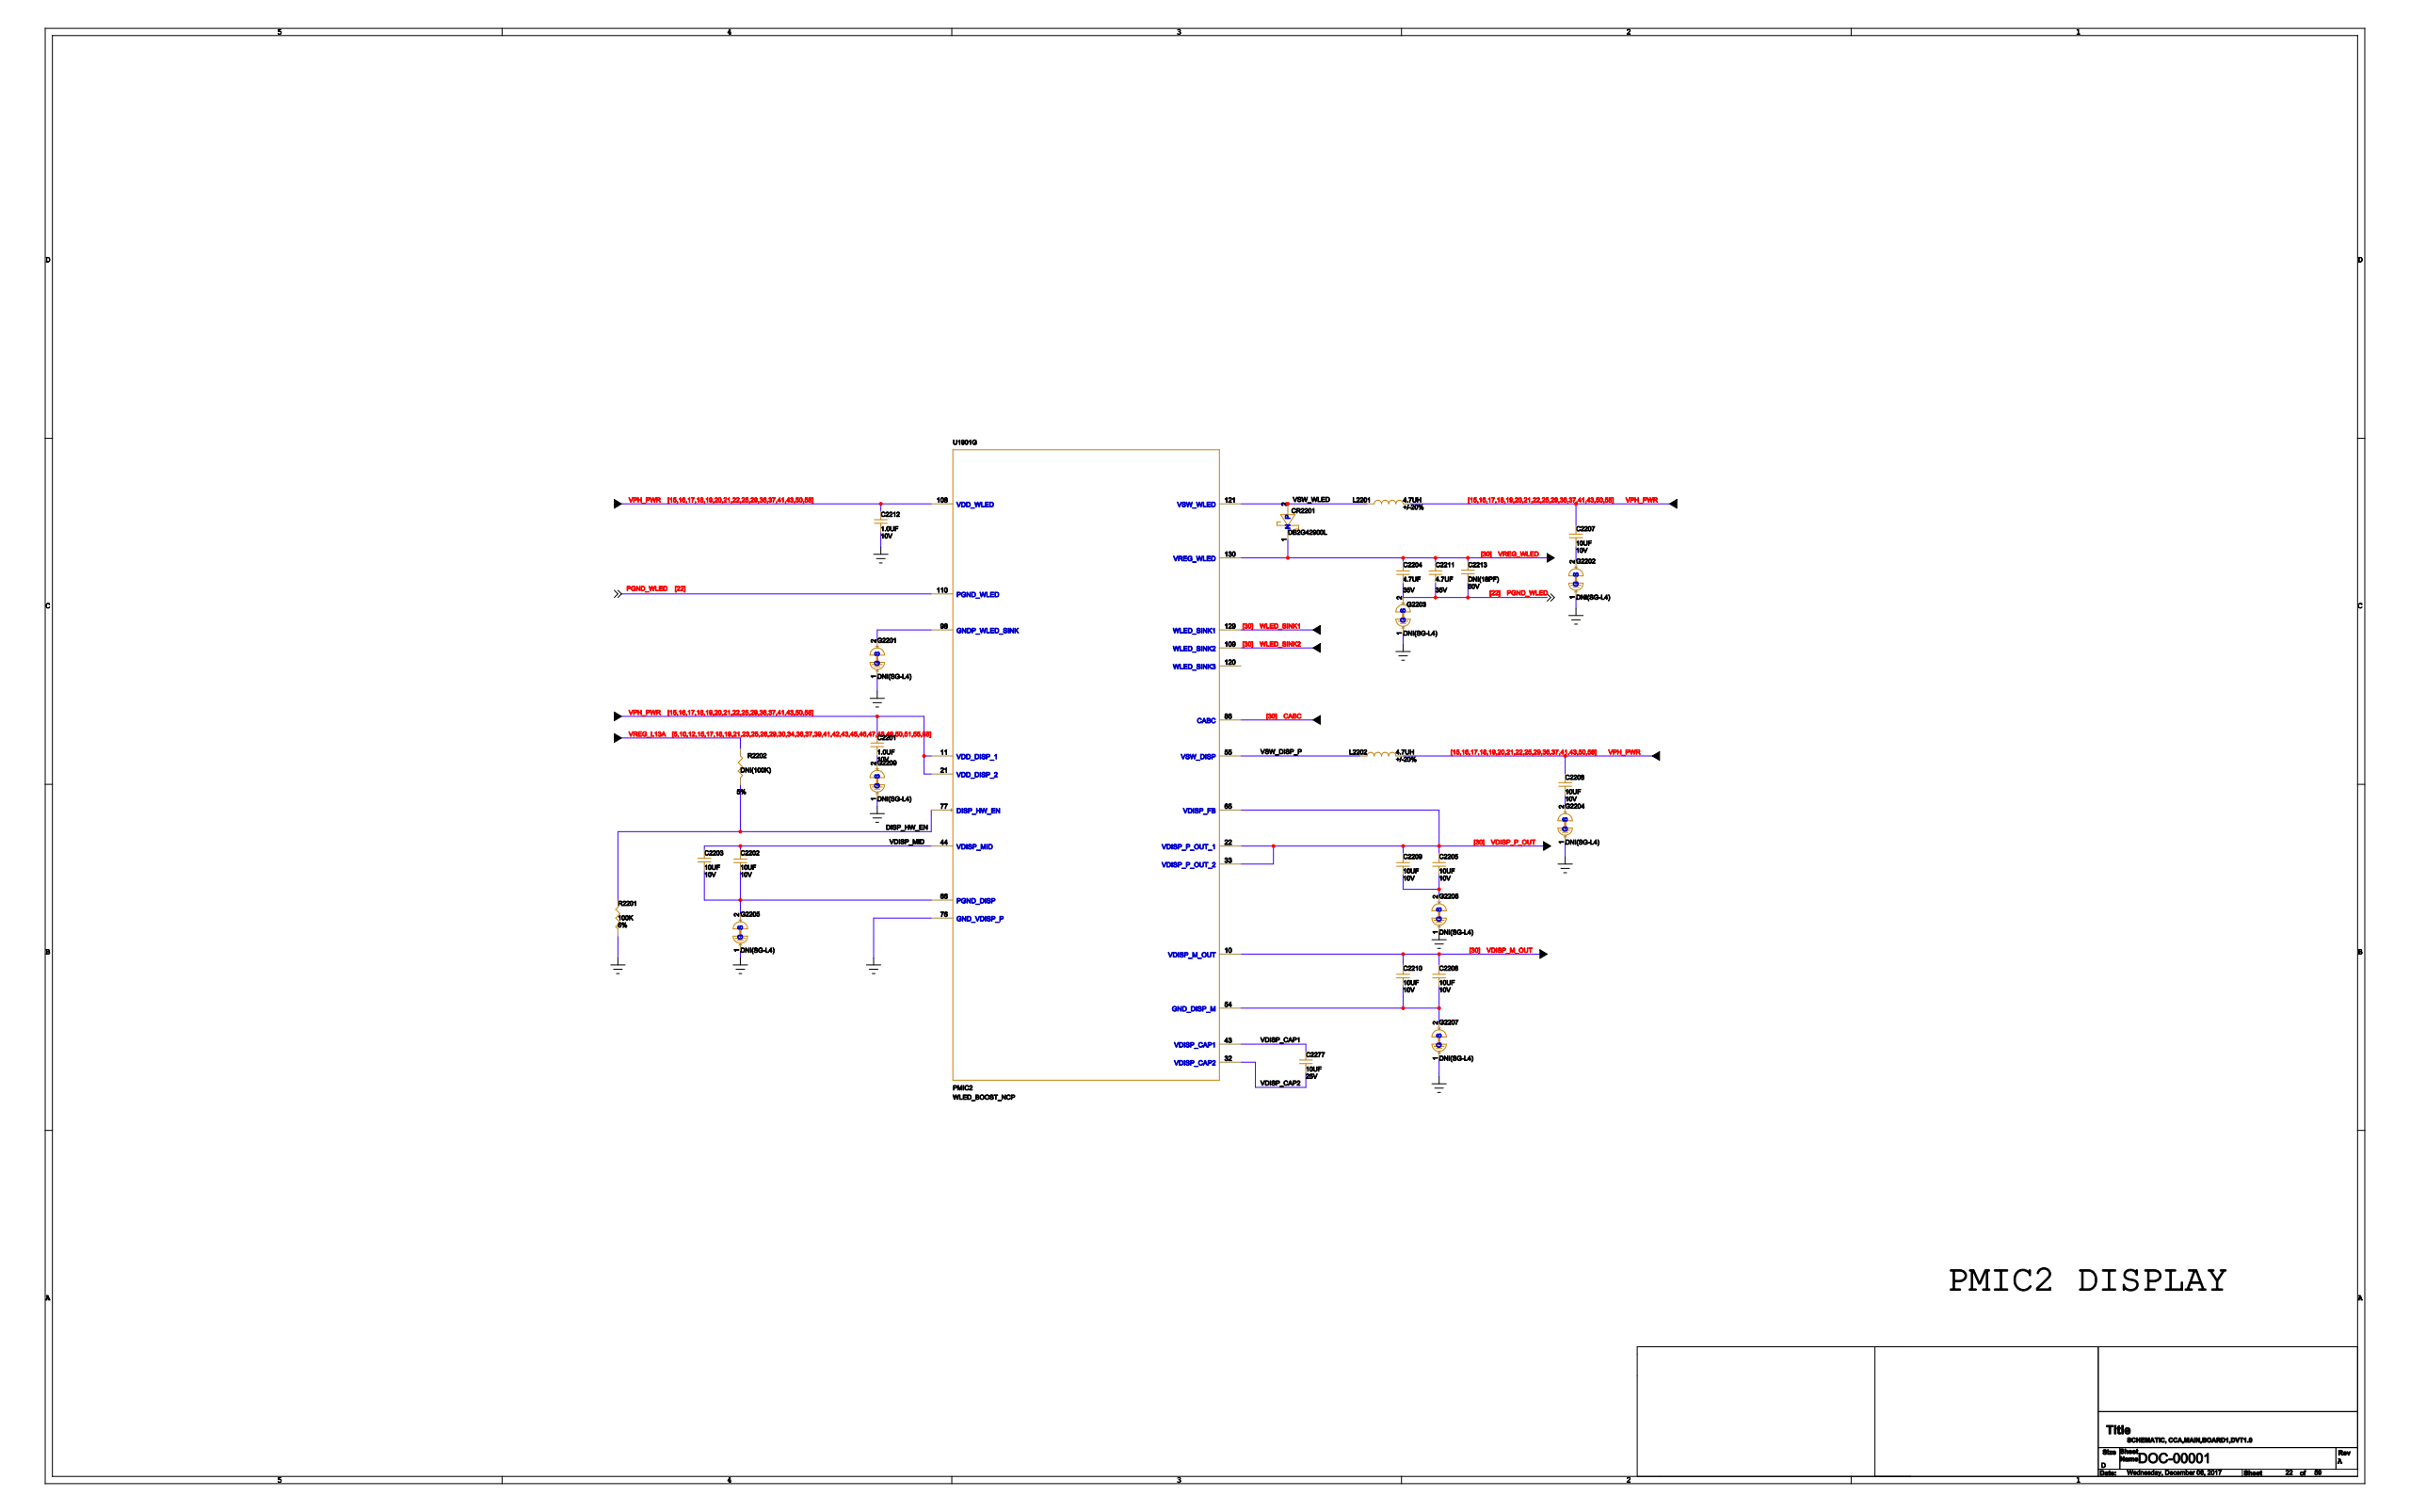Circuit board | KiCad | 1657 parts | 1365 nets | one sheet of the schematic
Parts on this sheet (reference | value | footprint):
C2201
C2202
C2203
C2204
C2205
C2206
C2207
C2208
C2209
C2210
C2211
C2212
C2213
C2277
CR2201
G2201
G2202
G2203
G2204
G2205
G2207
G2208
G2209
L2201
L2202
R2201
R2202
U1901
Nets of these parts (net: part-pin ...):
GND: C2212-2 G2201-1 G2202-1 G2203-1 G2204-1 G2205-1 G2207-1 G2208-1 G2209-1 R2201-2 U1901-76
VREG_L13A: R2202-2
VPH_PWR: C2201-1 C2207-1 C2208-1 C2212-1 L2201-2 L2202-2 U1901-2 U1901-11 U1901-17 U1901-21 U1901-39 U1901-108
N42480060: C2208-2 G2204-2
N42479215: G2201-2 U1901-98
CABC: U1901-86
N48943271: C2201-2 G2209-2
N48942883: C2205-1 C2209-1 G2208-2
PGND_WLED: C2204-1 C2211-1 C2213-2 G2203-2 U1901-110
N42480185: C2202-1 C2203-2 G2205-2 U1901-66
VDISP_P_OUT: C2205-2 C2209-2 U1901-22 U1901-33 U1901-65
N41101049: C2206-1 C2210-1 G2207-2 U1901-54
VDISP_M_OUT: C2206-2 C2210-2 U1901-10
WLED_SINK2: U1901-109
VREG_WLED: C2204-2 C2211-2 C2213-1 CR2201-1 U1901-130
N42479353: C2207-2 G2202-2
WLED_SINK1: U1901-129
DISP_HW_EN: R2201-1 R2202-1 U1901-77
VDISP_MID: C2202-2 C2203-1 U1901-44
VSW_WLED: CR2201-2 L2201-1 U1901-121
VDISP_CAP2: C2277-2 U1901-32
VDISP_CAP1: C2277-1 U1901-43
VSW_DISP_P: L2202-1 U1901-55
WLED_SINK3: U1901-120